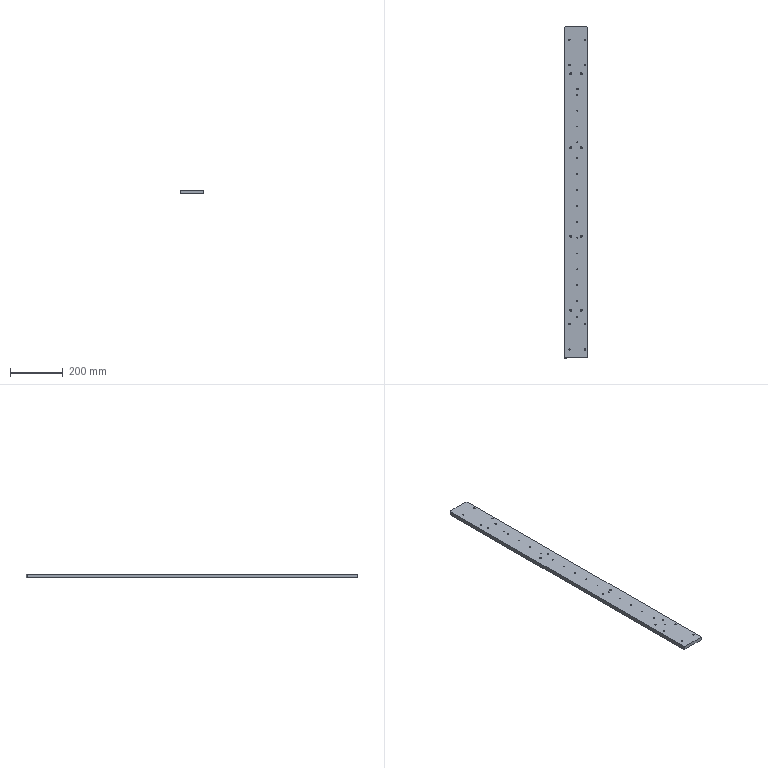Part | STEP file | PN_0029 | 1 solid | 140 faces | box 90 x 1255 x 15 mm | volume 1602482 mm3 | cylinder 94 | plane 26 | cone 20 | commonest cylinder face diameters 3.3 x30 5 x22 6.6 x16 11 x16 2.5 x8 10 x2